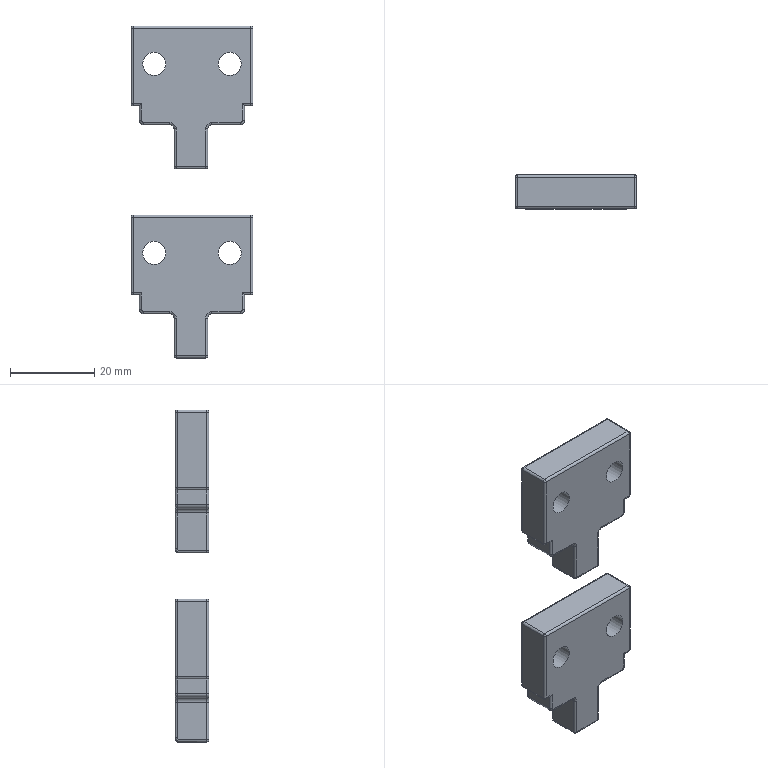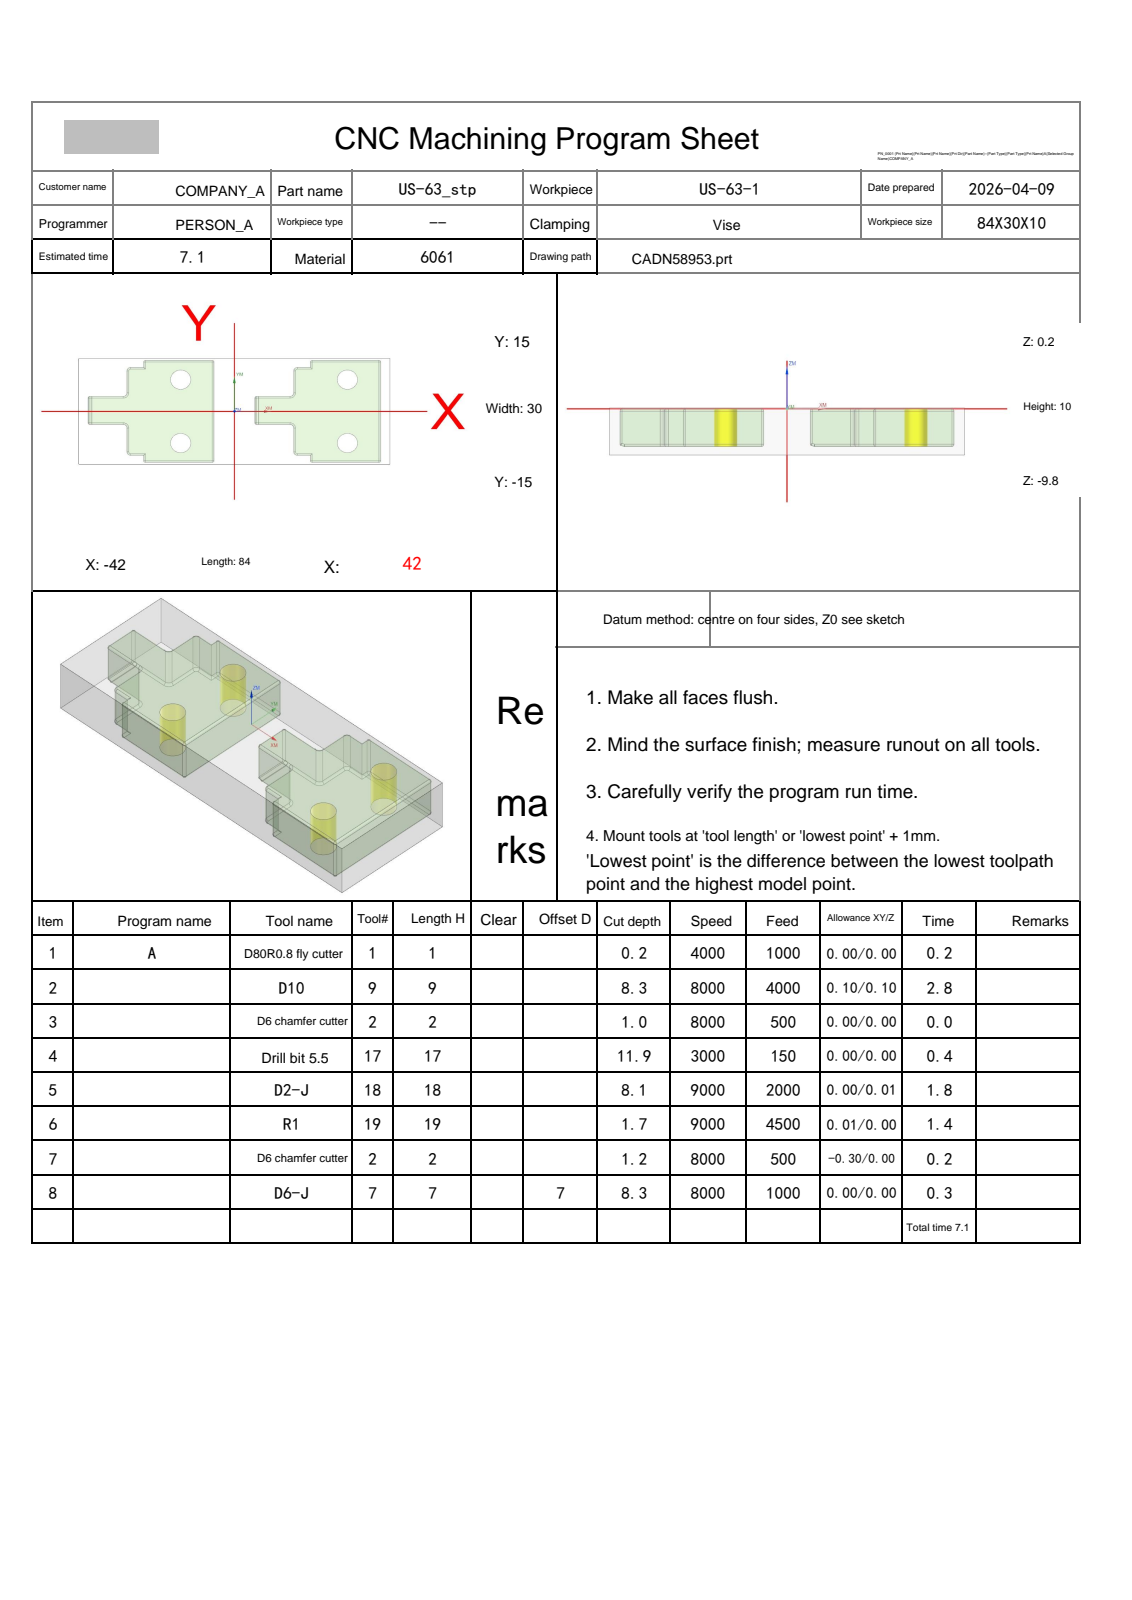NC program | NX | posted by the shop | part box 29 x 8 x 79 mm
Lines 34 to 1139 of 24039:
N2 T09 M06
(D10  D=10. R=0. H=09 ce=0.10 di=0.10)
G00 G90 G54 X12.55 Y-27. M03 S8000
G43 H09 Z10.2
M08
Z.724
G01 Z-.476 F4000.
Y-22.5
G03 X5.55 Y-15.5 I-7. J0.0
G01 X.837
G02 X-2.395 Y-20. I-6.837 J1.5
G01 X-27.605
G02 X-28.961 Y-18.938 I3.605 J6.
X-34.344 Y-15.5 I.961 J7.438
G01 X-42.
G02 X-42.5 Y-15. I0.0 J.5
G01 Y-10.535
G02 X-41.5 Y-9.535 I1. J0.0
X-41.214 Y-9.576 I0.0 J-1.
G01 X-39.39 Y-10.12
G03 X-38.298 Y-10.28 I1.092 J3.664
X-37.744 Y-10.239 I0.0 J3.824
G01 X-37.701 Y-10.236
X-35.798
G02 X-35.5 Y-10.535 I-.001 J-.3
G01 Y-10.701
G02 X-35.798 Y-11. I-.3 J.001
G01 X-37.701
X-37.79 Y-11.028
X-37.852 Y-10.958
G03 X-38.36 Y-10.82 I-.508 J-.862
X-38.599 Y-10.849 I0.0 J-1.
G01 X-41.26 Y-11.506
G02 X-41.5 Y-11.535 I-.24 J.971
X-42.5 Y-10.535 I0.0 J1.
G01 Y-9.298
G02 X-46. Y-3.236 I3.5 J6.062
G01 X-45.999 Y3.814
G02 X-42.5 Y9.825 I6.999 J-.05
G01 Y15.
G02 X-42. Y15.5 I.5 J0.0
G01 X-34.344
G02 X-28.961 Y18.938 I6.344 J-4.
X-27.605 Y20. I4.961 J-4.938
G01 X-2.395
G02 X.837 Y15.5 I-3.605 J-6.
G01 X4.477
G02 X5.477 Y14.5 I0.0 J-1.
X5.435 Y14.214 I-1. J0.0
G01 X4.831 Y12.187
G03 X4.667 Y11.066 I3.761 J-1.121
X4.675 Y10.813 I3.924 J0.0
G01 X4.676 Y10.8
G02 X4.519 Y10.605 I-.2 J0.0
G03 X2.089 Y9.569 I1.481 J-6.841
G02 X1.7 Y9.45 I-.39 J.582
X1. Y10.149 I0.0 J.7
G01 Y10.302
G02 X1.621 Y10.996 I.7 J-.002
G03 X2.454 Y11.666 I-.113 J.994
G01 X3.53 Y14.823
G02 X4.477 Y15.5 I.946 J-.323
G01 X10.656
G02 X16.039 Y18.938 I6.344 J-4.
X17.395 Y20. I4.961 J-4.938
G01 X42.
G02 X42.681 Y19.953 I0.0 J-5.
X46. Y14. I-3.681 J-5.953
G01 Y-14.
G02 X42.681 Y-19.953 I-7. J0.0
X42. Y-20. I-.681 J4.953
G01 X17.395
G02 X16.039 Y-18.938 I3.605 J6.
X10.656 Y-15.5 I.961 J7.438
G01 X.837
G02 X.77 Y-15.779 I-6.837 J1.5
X.417 Y-16.051 I-.353 J.093
X.052 Y-15.687 I0.0 J.365
G01 X.063 Y-15.596
X1.196 Y-11.178
G03 X1.223 Y-10.961 I-.844 J.216
X1.113 Y-10.538 I-.871 J0.0
G02 X1.003 Y-10.173 I.786 J.438
G03 X.812 Y-9.897 I-.335 J-.028
G01 X.2 Y-9.607
X.02 Y-9.566
G03 X-.4 Y-9.986 I0.0 J-.42
G01 Y-14.
G02 X-6. Y-19.6 I-5.6 J0.0
G01 X-24.
G02 X-28.295 Y-17.592 I0.0 J5.6
X-34.1 Y-11.5 I.295 J6.092
G01 Y-8.836
X-39.
G02 X-44.6 Y-3.236 I0.0 J5.6
G01 X-44.599 Y3.804
G02 X-39. Y9.363 I5.599 J-.04
G01 X-34.1
Y11.5
G02 X-28.295 Y17.592 I6.1 J0.0
X-24. Y19.6 I4.295 J-3.592
G01 X-6.
G02 X-.4 Y14. I0.0 J-5.6
G01 Y-9.986
G03 X.02 Y-10.406 I.42 J0.0
G01 X.2 Y-10.366
X.799 Y-10.081
G03 X1.019 Y-9.803 I-.172 J.361
G02 X1.9 Y-9.088 I.881 J-.186
X2.365 Y-9.218 I0.0 J-.9
G03 X6. Y-10.236 I3.635 J5.982
G01 X9.202
G02 X9.484 Y-10.437 I-.001 J-.3
G03 X9.885 Y-10.884 I.735 J.257
G01 X10.3 Y-11.081
X10.48 Y-11.121
G03 X10.9 Y-10.701 I0.0 J.42
G01 Y-8.836
X6.
G02 X.4 Y-3.236 I0.0 J5.6
G01 Y3.764
G02 X6. Y9.363 I5.6 J0.0
G01 X10.9
Y11.5
G02 X16.705 Y17.592 I6.1 J0.0
X21. Y19.6 I4.295 J-3.592
G01 X39.
G02 X44.6 Y14. I0.0 J-5.6
G01 Y-14.
G02 X39. Y-19.6 I-5.6 J0.0
G01 X21.
G02 X16.705 Y-17.592 I0.0 J5.6
X10.9 Y-11.5 I.295 J6.092
G01 Y-10.701
G03 X10.48 Y-10.281 I-.42 J0.0
G01 X10.3 Y-10.322
X9.669 Y-10.621
G03 X9.475 Y-10.821 I.172 J-.361
G02 X9.202 Y-11. I-.275 J.121
G01 X1.898
X1.724 Y-10.983
G02 X1.285 Y-10.757 I.176 J.883
G01 Z.724
G00 Z3.
G01 X12.55 Y-27. F6000.
G00 Z.247
G01 Z-.953 F4000.
Y-22.5
G03 X5.55 Y-15.5 I-7. J0.0
G01 X.837
G02 X-2.394 Y-20. I-6.837 J1.5
G01 X-27.606
G02 X-28.961 Y-18.938 I3.606 J6.
X-34.344 Y-15.5 I.961 J7.438
G01 X-42.
G02 X-42.5 Y-15. I0.0 J.5
G01 Y-10.535
G02 X-41.5 Y-9.535 I1. J0.0
X-41.214 Y-9.577 I0.0 J-1.
G01 X-39.39 Y-10.121
G03 X-38.298 Y-10.28 I1.092 J3.663
X-37.744 Y-10.24 I0.0 J3.823
G01 X-37.701 Y-10.236
X-35.799
G02 X-35.5 Y-10.535 I-.001 J-.3
G01 Y-10.701
G02 X-35.799 Y-11. I-.3 J.001
G01 X-37.701
X-37.79 Y-11.028
X-37.852 Y-10.958
G03 X-38.36 Y-10.82 I-.508 J-.862
X-38.599 Y-10.849 I0.0 J-1.
G01 X-41.26 Y-11.506
G02 X-41.5 Y-11.535 I-.24 J.971
X-42.5 Y-10.535 I0.0 J1.
G01 Y-9.299
G02 X-46. Y-3.236 I3.5 J6.062
G01 Y3.764
G02 X-42.5 Y9.826 I7. J0.0
G01 Y15.
G02 X-42. Y15.5 I.5 J0.0
G01 X-34.344
G02 X-28.961 Y18.938 I6.344 J-4.
X-27.606 Y20. I4.961 J-4.938
G01 X-2.394
G02 X.837 Y15.5 I-3.606 J-6.
G01 X4.475
G02 X5.475 Y14.5 I0.0 J-1.
X5.433 Y14.214 I-1. J0.0
G01 X4.828 Y12.187
G03 X4.665 Y11.067 I3.758 J-1.12
X4.673 Y10.813 I3.922 J0.0
G01 X4.674 Y10.8
G02 X4.517 Y10.605 I-.2 J0.0
G03 X2.09 Y9.57 I1.483 J-6.841
G02 X1.7 Y9.451 I-.39 J.582
X1. Y10.149 I0.0 J.7
G01 Y10.302
G02 X1.62 Y10.995 I.7 J-.002
G03 X2.452 Y11.666 I-.115 J.993
G01 X3.528 Y14.823
G02 X4.475 Y15.5 I.946 J-.323
G01 X10.656
G02 X16.039 Y18.938 I6.344 J-4.
X17.394 Y20. I4.961 J-4.938
G01 X42.
G02 X42.682 Y19.953 I0.0 J-5.
X46. Y14. I-3.682 J-5.953
G01 Y-14.
G02 X42.682 Y-19.953 I-7. J0.0
X42. Y-20. I-.682 J4.953
G01 X17.394
G02 X16.039 Y-18.938 I3.606 J6.
X10.656 Y-15.5 I.961 J7.438
G01 X.837
G02 X.77 Y-15.78 I-6.837 J1.5
X.417 Y-16.052 I-.353 J.093
X.052 Y-15.687 I0.0 J.365
G01 X.064 Y-15.596
X1.197 Y-11.178
G03 X1.224 Y-10.962 I-.844 J.216
X1.114 Y-10.538 I-.871 J0.0
G02 X1.003 Y-10.174 I.786 J.438
G03 X.813 Y-9.898 I-.334 J-.028
G01 X.2 Y-9.608
X.02 Y-9.567
G03 X-.4 Y-9.987 I0.0 J-.42
G01 Y-14.
G02 X-6. Y-19.6 I-5.6 J0.0
G01 X-24.
G02 X-28.296 Y-17.593 I0.0 J5.6
X-34.1 Y-11.5 I.296 J6.093
G01 Y-8.836
X-39.
G02 X-44.6 Y-3.236 I0.0 J5.6
G01 Y3.764
G02 X-39. Y9.364 I5.6 J0.0
G01 X-34.1
Y11.5
G02 X-28.296 Y17.593 I6.1 J0.0
X-24. Y19.6 I4.296 J-3.593
G01 X-6.
G02 X-.4 Y14. I0.0 J-5.6
G01 Y-9.987
G03 X.02 Y-10.407 I.42 J0.0
G01 X.2 Y-10.367
X.8 Y-10.082
G03 X1.019 Y-9.804 I-.172 J.361
G02 X1.9 Y-9.089 I.881 J-.186
X2.366 Y-9.219 I0.0 J-.9
G03 X6. Y-10.236 I3.634 J5.983
G01 X9.201
G02 X9.483 Y-10.437 I-.001 J-.3
G03 X9.884 Y-10.883 I.735 J.258
G01 X10.3 Y-11.081
X10.48 Y-11.121
G03 X10.9 Y-10.701 I0.0 J.42
G01 Y-8.836
X6.
G02 X.4 Y-3.236 I0.0 J5.6
G01 Y3.764
G02 X6. Y9.364 I5.6 J0.0
G01 X10.9
Y11.5
G02 X16.704 Y17.593 I6.1 J0.0
X21. Y19.6 I4.296 J-3.593
G01 X39.
G02 X44.6 Y14. I0.0 J-5.6
G01 Y-14.
G02 X39. Y-19.6 I-5.6 J0.0
G01 X21.
G02 X16.704 Y-17.593 I0.0 J5.6
X10.9 Y-11.5 I.296 J6.093
G01 Y-10.701
G03 X10.48 Y-10.281 I-.42 J0.0
G01 X10.3 Y-10.322
X9.669 Y-10.621
G03 X9.475 Y-10.821 I.172 J-.361
G02 X9.201 Y-11. I-.275 J.121
G01 X1.898
X1.724 Y-10.983
G02 X1.285 Y-10.757 I.176 J.883
G01 Z.247
G00 Z2.524
G01 X12.55 Y-27. F6000.
G00 Z-.229
G01 Z-1.429 F4000.
Y-22.5
G03 X5.55 Y-15.5 I-7. J0.0
G01 X.837
G02 X-2.394 Y-20. I-6.837 J1.5
G01 X-27.606
G02 X-28.961 Y-18.938 I3.606 J6.
X-34.344 Y-15.5 I.961 J7.438
G01 X-42.
G02 X-42.5 Y-15. I0.0 J.5
G01 Y-10.535
G02 X-41.5 Y-9.535 I1. J0.0
X-41.214 Y-9.577 I0.0 J-1.
G01 X-39.39 Y-10.121
G03 X-38.298 Y-10.28 I1.092 J3.663
X-37.744 Y-10.24 I0.0 J3.822
G01 X-37.701 Y-10.236
X-35.799
G02 X-35.5 Y-10.535 I-.001 J-.3
G01 Y-10.701
G02 X-35.799 Y-11. I-.3 J.001
G01 X-37.701
X-37.79 Y-11.028
X-37.852 Y-10.958
G03 X-38.36 Y-10.82 I-.507 J-.862
X-38.599 Y-10.849 I0.0 J-1.
G01 X-41.26 Y-11.506
G02 X-41.5 Y-11.535 I-.24 J.971
X-42.5 Y-10.535 I0.0 J1.
G01 Y-9.299
G02 X-46. Y-3.236 I3.5 J6.062
G01 Y3.764
G02 X-42.5 Y9.826 I7. J0.0
G01 Y15.
G02 X-42. Y15.5 I.5 J0.0
G01 X-34.344
G02 X-28.961 Y18.938 I6.344 J-4.
X-27.606 Y20. I4.961 J-4.938
G01 X-2.394
G02 X.837 Y15.5 I-3.606 J-6.
G01 X4.475
G02 X5.475 Y14.5 I0.0 J-1.
X5.433 Y14.214 I-1. J0.0
G01 X4.828 Y12.186
G03 X4.665 Y11.066 I3.758 J-1.12
X4.673 Y10.813 I3.922 J0.0
G01 X4.674 Y10.8
G02 X4.517 Y10.605 I-.2 J0.0
G03 X2.089 Y9.569 I1.483 J-6.841
G02 X1.7 Y9.451 I-.389 J.582
X1. Y10.149 I0.0 J.7
G01 Y10.302
G02 X1.62 Y10.995 I.7 J-.002
G03 X2.452 Y11.666 I-.115 J.993
G01 X3.528 Y14.823
G02 X4.475 Y15.5 I.946 J-.323
G01 X10.656
G02 X16.039 Y18.938 I6.344 J-4.
X17.394 Y20. I4.961 J-4.938
G01 X42.
G02 X42.682 Y19.953 I0.0 J-5.
X46. Y14. I-3.682 J-5.953
G01 Y-14.
G02 X42.682 Y-19.953 I-7. J0.0
X42. Y-20. I-.682 J4.953
G01 X17.394
G02 X16.039 Y-18.938 I3.606 J6.
X10.656 Y-15.5 I.961 J7.438
G01 X.837
G02 X.77 Y-15.78 I-6.837 J1.5
X.417 Y-16.052 I-.353 J.093
X.052 Y-15.687 I0.0 J.365
G01 X.064 Y-15.596
X1.197 Y-11.178
G03 X1.224 Y-10.962 I-.844 J.216
X1.114 Y-10.538 I-.871 J0.0
G02 X1.003 Y-10.174 I.786 J.438
G03 X.813 Y-9.898 I-.334 J-.028
G01 X.2 Y-9.608
X.02 Y-9.567
G03 X-.4 Y-9.987 I0.0 J-.42
G01 Y-14.
G02 X-6. Y-19.6 I-5.6 J0.0
G01 X-24.
G02 X-28.296 Y-17.593 I0.0 J5.6
X-34.1 Y-11.5 I.296 J6.093
G01 Y-8.836
X-39.
G02 X-44.6 Y-3.236 I0.0 J5.6
G01 Y3.764
G02 X-39. Y9.364 I5.6 J0.0
G01 X-34.1
Y11.5
G02 X-28.296 Y17.593 I6.1 J0.0
X-24. Y19.6 I4.296 J-3.593
G01 X-6.
G02 X-.4 Y14. I0.0 J-5.6
G01 Y-9.987
G03 X.02 Y-10.407 I.42 J0.0
G01 X.2 Y-10.366
X.8 Y-10.082
G03 X1.019 Y-9.803 I-.172 J.361
G02 X1.9 Y-9.089 I.881 J-.186
X2.365 Y-9.219 I0.0 J-.9
G03 X6. Y-10.236 I3.635 J5.982
G01 X9.201
G02 X9.483 Y-10.437 I-.001 J-.3
G03 X9.884 Y-10.884 I.735 J.258
G01 X10.3 Y-11.081
X10.48 Y-11.121
G03 X10.9 Y-10.701 I0.0 J.42
G01 Y-8.836
X6.
G02 X.4 Y-3.236 I0.0 J5.6
G01 Y3.764
G02 X6. Y9.364 I5.6 J0.0
G01 X10.9
Y11.5
G02 X16.704 Y17.593 I6.1 J0.0
X21. Y19.6 I4.296 J-3.593
G01 X39.
G02 X44.6 Y14. I0.0 J-5.6
G01 Y-14.
G02 X39. Y-19.6 I-5.6 J0.0
G01 X21.
G02 X16.704 Y-17.593 I0.0 J5.6
X10.9 Y-11.5 I.296 J6.093
G01 Y-10.701
G03 X10.48 Y-10.281 I-.42 J0.0
G01 X10.3 Y-10.322
X9.669 Y-10.621
G03 X9.475 Y-10.821 I.172 J-.361
G02 X9.201 Y-11. I-.275 J.121
G01 X1.898
X1.724 Y-10.983
G02 X1.285 Y-10.757 I.176 J.883
G01 Z-.229
G00 Z2.047
G01 X12.55 Y-27. F6000.
G00 Z-.706
G01 Z-1.906 F4000.
Y-22.5
G03 X5.55 Y-15.5 I-7. J0.0
G01 X.837
G02 X-2.394 Y-20. I-6.837 J1.5
G01 X-27.606
G02 X-28.961 Y-18.938 I3.606 J6.
X-34.344 Y-15.5 I.961 J7.438
G01 X-42.
G02 X-42.5 Y-15. I0.0 J.5
G01 Y-10.535
G02 X-41.5 Y-9.535 I1. J0.0
X-41.214 Y-9.577 I0.0 J-1.
G01 X-39.39 Y-10.121
G03 X-38.298 Y-10.28 I1.092 J3.663
X-37.744 Y-10.24 I0.0 J3.823
G01 X-37.701 Y-10.236
X-35.799
G02 X-35.5 Y-10.535 I-.001 J-.3
G01 Y-10.701
G02 X-35.799 Y-11. I-.3 J.001
G01 X-37.701
X-37.79 Y-11.028
X-37.852 Y-10.958
G03 X-38.36 Y-10.82 I-.508 J-.862
X-38.599 Y-10.849 I0.0 J-1.
G01 X-41.26 Y-11.506
G02 X-41.5 Y-11.535 I-.24 J.971
X-42.5 Y-10.535 I0.0 J1.
G01 Y-9.299
G02 X-46. Y-3.236 I3.5 J6.062
G01 Y3.764
G02 X-42.5 Y9.826 I7. J0.0
G01 Y15.
G02 X-42. Y15.5 I.5 J0.0
G01 X-34.344
G02 X-28.961 Y18.938 I6.344 J-4.
X-27.606 Y20. I4.961 J-4.938
G01 X-2.394
G02 X.837 Y15.5 I-3.606 J-6.
G01 X4.475
G02 X5.475 Y14.5 I0.0 J-1.
X5.433 Y14.214 I-1. J0.0
G01 X4.828 Y12.187
G03 X4.665 Y11.067 I3.758 J-1.12
X4.673 Y10.813 I3.922 J0.0
G01 X4.674 Y10.8
G02 X4.517 Y10.605 I-.2 J0.0
G03 X2.09 Y9.57 I1.483 J-6.841
G02 X1.7 Y9.451 I-.39 J.582
X1. Y10.149 I0.0 J.7
G01 Y10.302
G02 X1.62 Y10.995 I.7 J-.002
G03 X2.452 Y11.666 I-.115 J.993
G01 X3.528 Y14.823
G02 X4.475 Y15.5 I.946 J-.323
G01 X10.656
G02 X16.039 Y18.938 I6.344 J-4.
X17.394 Y20. I4.961 J-4.938
G01 X42.
G02 X42.682 Y19.953 I0.0 J-5.
X46. Y14. I-3.682 J-5.953
G01 Y-14.
G02 X42.682 Y-19.953 I-7. J0.0
X42. Y-20. I-.682 J4.953
G01 X17.394
G02 X16.039 Y-18.938 I3.606 J6.
X10.656 Y-15.5 I.961 J7.438
G01 X.837
G02 X.77 Y-15.78 I-6.837 J1.5
X.417 Y-16.052 I-.353 J.093
X.052 Y-15.687 I0.0 J.365
G01 X.064 Y-15.596
X1.197 Y-11.178
G03 X1.224 Y-10.962 I-.844 J.216
X1.114 Y-10.538 I-.871 J0.0
G02 X1.003 Y-10.174 I.786 J.438
G03 X.813 Y-9.898 I-.334 J-.028
G01 X.2 Y-9.608
X.02 Y-9.567
G03 X-.4 Y-9.987 I0.0 J-.42
G01 Y-14.
G02 X-6. Y-19.6 I-5.6 J0.0
G01 X-24.
G02 X-28.296 Y-17.593 I0.0 J5.6
X-34.1 Y-11.5 I.296 J6.093
G01 Y-8.836
X-39.
G02 X-44.6 Y-3.236 I0.0 J5.6
G01 Y3.764
G02 X-39. Y9.364 I5.6 J0.0
G01 X-34.1
Y11.5
G02 X-28.296 Y17.593 I6.1 J0.0
X-24. Y19.6 I4.296 J-3.593
G01 X-6.
G02 X-.4 Y14. I0.0 J-5.6
G01 Y-9.987
G03 X.02 Y-10.407 I.42 J0.0
G01 X.2 Y-10.367
X.8 Y-10.082
G03 X1.019 Y-9.804 I-.172 J.361
G02 X1.9 Y-9.089 I.881 J-.186
X2.366 Y-9.219 I0.0 J-.9
G03 X6. Y-10.236 I3.634 J5.983
G01 X9.201
G02 X9.483 Y-10.437 I-.001 J-.3
G03 X9.884 Y-10.883 I.735 J.258
G01 X10.3 Y-11.081
X10.48 Y-11.121
G03 X10.9 Y-10.701 I0.0 J.42
G01 Y-8.836
X6.
G02 X.4 Y-3.236 I0.0 J5.6
G01 Y3.764
G02 X6. Y9.364 I5.6 J0.0
G01 X10.9
Y11.5
G02 X16.704 Y17.593 I6.1 J0.0
X21. Y19.6 I4.296 J-3.593
G01 X39.
G02 X44.6 Y14. I0.0 J-5.6
G01 Y-14.
G02 X39. Y-19.6 I-5.6 J0.0
G01 X21.
G02 X16.704 Y-17.593 I0.0 J5.6
X10.9 Y-11.5 I.296 J6.093
G01 Y-10.701
G03 X10.48 Y-10.281 I-.42 J0.0
G01 X10.3 Y-10.322
X9.669 Y-10.621
G03 X9.475 Y-10.821 I.172 J-.361
G02 X9.201 Y-11. I-.275 J.121
G01 X1.898
X1.724 Y-10.983
G02 X1.285 Y-10.757 I.176 J.883
G01 Z-.706
G00 Z1.571
G01 X12.55 Y-27. F6000.
G00 Z-1.182
G01 Z-2.382 F4000.
Y-22.5
G03 X5.55 Y-15.5 I-7. J0.0
G01 X.837
G02 X-2.394 Y-20. I-6.837 J1.5
G01 X-27.606
G02 X-28.961 Y-18.938 I3.606 J6.
X-34.344 Y-15.5 I.961 J7.438
G01 X-42.
G02 X-42.5 Y-15. I0.0 J.5
G01 Y-10.535
G02 X-41.5 Y-9.535 I1. J0.0
X-41.214 Y-9.577 I0.0 J-1.
G01 X-39.39 Y-10.121
G03 X-38.298 Y-10.28 I1.092 J3.663
X-37.744 Y-10.24 I0.0 J3.822
G01 X-37.701 Y-10.236
X-35.799
G02 X-35.5 Y-10.535 I-.001 J-.3
G01 Y-10.701
G02 X-35.799 Y-11. I-.3 J.001
G01 X-37.701
X-37.79 Y-11.028
X-37.852 Y-10.958
G03 X-38.36 Y-10.82 I-.507 J-.862
X-38.599 Y-10.849 I0.0 J-1.
G01 X-41.26 Y-11.506
G02 X-41.5 Y-11.535 I-.24 J.971
X-42.5 Y-10.535 I0.0 J1.
G01 Y-9.299
G02 X-46. Y-3.236 I3.5 J6.062
G01 Y3.764
G02 X-42.5 Y9.826 I7. J0.0
G01 Y15.
G02 X-42. Y15.5 I.5 J0.0
G01 X-34.344
G02 X-28.961 Y18.938 I6.344 J-4.
X-27.606 Y20. I4.961 J-4.938
G01 X-2.394
G02 X.837 Y15.5 I-3.606 J-6.
G01 X4.475
G02 X5.475 Y14.5 I0.0 J-1.
X5.433 Y14.214 I-1. J0.0
G01 X4.828 Y12.186
G03 X4.665 Y11.066 I3.758 J-1.12
X4.673 Y10.813 I3.922 J0.0
G01 X4.674 Y10.8
G02 X4.517 Y10.605 I-.2 J0.0
G03 X2.089 Y9.569 I1.483 J-6.841
G02 X1.7 Y9.451 I-.389 J.582
X1. Y10.149 I0.0 J.7
G01 Y10.302
G02 X1.62 Y10.995 I.7 J-.002
G03 X2.452 Y11.666 I-.115 J.993
G01 X3.528 Y14.823
G02 X4.475 Y15.5 I.946 J-.323
G01 X10.656
G02 X16.039 Y18.938 I6.344 J-4.
X17.394 Y20. I4.961 J-4.938
G01 X42.
G02 X42.682 Y19.953 I0.0 J-5.
X46. Y14. I-3.682 J-5.953
G01 Y-14.
G02 X42.682 Y-19.953 I-7. J0.0
X42. Y-20. I-.682 J4.953
G01 X17.394
G02 X16.039 Y-18.938 I3.606 J6.
X10.656 Y-15.5 I.961 J7.438
G01 X.837
G02 X.77 Y-15.78 I-6.837 J1.5
X.417 Y-16.052 I-.353 J.093
X.052 Y-15.687 I0.0 J.365
G01 X.064 Y-15.596
X1.197 Y-11.178
G03 X1.224 Y-10.962 I-.844 J.216
X1.114 Y-10.538 I-.871 J0.0
G02 X1.003 Y-10.174 I.786 J.438
G03 X.813 Y-9.898 I-.334 J-.028
G01 X.2 Y-9.608
X.02 Y-9.567
G03 X-.4 Y-9.987 I0.0 J-.42
G01 Y-14.
G02 X-6. Y-19.6 I-5.6 J0.0
G01 X-24.
G02 X-28.296 Y-17.593 I0.0 J5.6
X-34.1 Y-11.5 I.296 J6.093
G01 Y-8.836
X-39.
G02 X-44.6 Y-3.236 I0.0 J5.6
G01 Y3.764
G02 X-39. Y9.364 I5.6 J0.0
G01 X-34.1
Y11.5
G02 X-28.296 Y17.593 I6.1 J0.0
X-24. Y19.6 I4.296 J-3.593
G01 X-6.
G02 X-.4 Y14. I0.0 J-5.6
G01 Y-9.987
G03 X.02 Y-10.407 I.42 J0.0
G01 X.2 Y-10.366
X.8 Y-10.082
G03 X1.019 Y-9.803 I-.172 J.361
G02 X1.9 Y-9.089 I.881 J-.186
X2.365 Y-9.219 I0.0 J-.9
G03 X6. Y-10.236 I3.635 J5.982
G01 X9.201
G02 X9.483 Y-10.437 I-.001 J-.3
G03 X9.884 Y-10.884 I.735 J.258
G01 X10.3 Y-11.081
X10.48 Y-11.121
G03 X10.9 Y-10.701 I0.0 J.42
G01 Y-8.836
X6.
G02 X.4 Y-3.236 I0.0 J5.6
G01 Y3.764
G02 X6. Y9.364 I5.6 J0.0
G01 X10.9
Y11.5
G02 X16.704 Y17.593 I6.1 J0.0
X21. Y19.6 I4.296 J-3.593
G01 X39.
G02 X44.6 Y14. I0.0 J-5.6
G01 Y-14.
G02 X39. Y-19.6 I-5.6 J0.0
G01 X21.
G02 X16.704 Y-17.593 I0.0 J5.6
X10.9 Y-11.5 I.296 J6.093
G01 Y-10.701
G03 X10.48 Y-10.281 I-.42 J0.0
G01 X10.3 Y-10.322
X9.669 Y-10.621
G03 X9.475 Y-10.821 I.172 J-.361
G02 X9.201 Y-11. I-.275 J.121
G01 X1.898
X1.724 Y-10.983
G02 X1.285 Y-10.757 I.176 J.883
G01 Z-1.182
G00 Z1.094
G01 X12.55 Y-27. F6000.
G00 Z-1.659
G01 Z-2.859 F4000.
Y-22.5
G03 X5.55 Y-15.5 I-7. J0.0
G01 X.837
G02 X-2.394 Y-20. I-6.837 J1.5
G01 X-27.606
G02 X-28.961 Y-18.938 I3.606 J6.
X-34.344 Y-15.5 I.961 J7.438
G01 X-42.
G02 X-42.5 Y-15. I0.0 J.5
G01 Y-10.535
G02 X-41.5 Y-9.535 I1. J0.0
X-41.214 Y-9.577 I0.0 J-1.
G01 X-39.39 Y-10.121
G03 X-38.298 Y-10.28 I1.092 J3.663
X-37.744 Y-10.24 I0.0 J3.823
G01 X-37.701 Y-10.236
X-35.799
G02 X-35.5 Y-10.535 I-.001 J-.3
G01 Y-10.701
G02 X-35.799 Y-11. I-.3 J.001
G01 X-37.701
X-37.79 Y-11.028
X-37.852 Y-10.958
G03 X-38.36 Y-10.82 I-.508 J-.862
X-38.599 Y-10.849 I0.0 J-1.
G01 X-41.26 Y-11.506
G02 X-41.5 Y-11.535 I-.24 J.971
X-42.5 Y-10.535 I0.0 J1.
G01 Y-9.299
G02 X-46. Y-3.236 I3.5 J6.062
G01 Y3.764
G02 X-42.5 Y9.826 I7. J0.0
G01 Y15.
G02 X-42. Y15.5 I.5 J0.0
G01 X-34.344
G02 X-28.961 Y18.938 I6.344 J-4.
X-27.606 Y20. I4.961 J-4.938
G01 X-2.394
G02 X.837 Y15.5 I-3.606 J-6.
G01 X4.475
G02 X5.475 Y14.5 I0.0 J-1.
X5.433 Y14.214 I-1. J0.0
G01 X4.828 Y12.187
G03 X4.665 Y11.067 I3.758 J-1.12
X4.673 Y10.813 I3.922 J0.0
G01 X4.674 Y10.8
G02 X4.517 Y10.605 I-.2 J0.0
G03 X2.09 Y9.57 I1.483 J-6.841
G02 X1.7 Y9.451 I-.39 J.582
X1. Y10.149 I0.0 J.7
G01 Y10.302
G02 X1.62 Y10.995 I.7 J-.002
G03 X2.452 Y11.666 I-.115 J.993
G01 X3.528 Y14.823
G02 X4.475 Y15.5 I.946 J-.323
G01 X10.656
G02 X16.039 Y18.938 I6.344 J-4.
X17.394 Y20. I4.961 J-4.938
G01 X42.
G02 X42.682 Y19.953 I0.0 J-5.
X46. Y14. I-3.682 J-5.953
G01 Y-14.
G02 X42.682 Y-19.953 I-7. J0.0
X42. Y-20. I-.682 J4.953
G01 X17.394
G02 X16.039 Y-18.938 I3.606 J6.
X10.656 Y-15.5 I.961 J7.438
G01 X.837
G02 X.77 Y-15.78 I-6.837 J1.5
X.417 Y-16.052 I-.353 J.093
X.052 Y-15.687 I0.0 J.365
G01 X.064 Y-15.596
X1.197 Y-11.178
G03 X1.224 Y-10.962 I-.844 J.216
X1.114 Y-10.538 I-.871 J0.0
G02 X1.003 Y-10.174 I.786 J.438
G03 X.813 Y-9.898 I-.334 J-.028
G01 X.2 Y-9.608
X.02 Y-9.567
G03 X-.4 Y-9.987 I0.0 J-.42
G01 Y-14.
G02 X-6. Y-19.6 I-5.6 J0.0
G01 X-24.
G02 X-28.296 Y-17.593 I0.0 J5.6
X-34.1 Y-11.5 I.296 J6.093
G01 Y-8.836
X-39.
G02 X-44.6 Y-3.236 I0.0 J5.6
G01 Y3.764
G02 X-39. Y9.364 I5.6 J0.0
G01 X-34.1
Y11.5
G02 X-28.296 Y17.593 I6.1 J0.0
X-24. Y19.6 I4.296 J-3.593
G01 X-6.
G02 X-.4 Y14. I0.0 J-5.6
G01 Y-9.987
G03 X.02 Y-10.407 I.42 J0.0
G01 X.2 Y-10.367
X.8 Y-10.082
G03 X1.019 Y-9.804 I-.172 J.361
G02 X1.9 Y-9.089 I.881 J-.186
X2.366 Y-9.219 I0.0 J-.9
G03 X6. Y-10.236 I3.634 J5.983
G01 X9.201
G02 X9.483 Y-10.437 I-.001 J-.3
G03 X9.884 Y-10.883 I.735 J.258
G01 X10.3 Y-11.081
X10.48 Y-11.121
G03 X10.9 Y-10.701 I0.0 J.42
G01 Y-8.836
X6.
G02 X.4 Y-3.236 I0.0 J5.6
G01 Y3.764
G02 X6. Y9.364 I5.6 J0.0
G01 X10.9
Y11.5
G02 X16.704 Y17.593 I6.1 J0.0
X21. Y19.6 I4.296 J-3.593
G01 X39.
G02 X44.6 Y14. I0.0 J-5.6
G01 Y-14.
G02 X39. Y-19.6 I-5.6 J0.0
G01 X21.
G02 X16.704 Y-17.593 I0.0 J5.6
X10.9 Y-11.5 I.296 J6.093
G01 Y-10.701
G03 X10.48 Y-10.281 I-.42 J0.0
G01 X10.3 Y-10.322
X9.669 Y-10.621
G03 X9.475 Y-10.821 I.172 J-.361
G02 X9.201 Y-11. I-.275 J.121
G01 X1.898
X1.724 Y-10.983
G02 X1.285 Y-10.757 I.176 J.883
G01 Z-1.659
G00 Z.618
G01 X12.55 Y-27. F6000.
G00 Z-2.135
G01 Z-3.335 F4000.
Y-22.5
G03 X5.55 Y-15.5 I-7. J0.0
G01 X.837
G02 X-2.394 Y-20. I-6.837 J1.5
G01 X-27.606
G02 X-28.961 Y-18.938 I3.606 J6.
X-34.344 Y-15.5 I.961 J7.438
G01 X-42.
G02 X-42.5 Y-15. I0.0 J.5
G01 Y-10.535
G02 X-41.5 Y-9.535 I1. J0.0
X-41.214 Y-9.577 I0.0 J-1.
G01 X-39.39 Y-10.121
G03 X-38.298 Y-10.28 I1.092 J3.663
X-37.744 Y-10.24 I0.0 J3.822
G01 X-37.701 Y-10.236
X-35.799
G02 X-35.5 Y-10.535 I-.001 J-.3
G01 Y-10.701
G02 X-35.799 Y-11. I-.3 J.001
G01 X-37.701
X-37.79 Y-11.028
X-37.852 Y-10.958
G03 X-38.36 Y-10.82 I-.507 J-.862
X-38.599 Y-10.849 I0.0 J-1.
G01 X-41.26 Y-11.506
G02 X-41.5 Y-11.535 I-.24 J.971
X-42.5 Y-10.535 I0.0 J1.
G01 Y-9.299
G02 X-46. Y-3.236 I3.5 J6.062
G01 Y3.764
G02 X-42.5 Y9.826 I7. J0.0
G01 Y15.
G02 X-42. Y15.5 I.5 J0.0
G01 X-34.344
G02 X-28.961 Y18.938 I6.344 J-4.
X-27.606 Y20. I4.961 J-4.938
G01 X-2.394
G02 X.837 Y15.5 I-3.606 J-6.
G01 X4.475
G02 X5.475 Y14.5 I0.0 J-1.
X5.433 Y14.214 I-1. J0.0
G01 X4.828 Y12.186
G03 X4.665 Y11.066 I3.758 J-1.12
X4.673 Y10.813 I3.922 J0.0
G01 X4.674 Y10.8
G02 X4.517 Y10.605 I-.2 J0.0
G03 X2.089 Y9.569 I1.483 J-6.841
G02 X1.7 Y9.451 I-.389 J.582
X1. Y10.149 I0.0 J.7
G01 Y10.302
G02 X1.62 Y10.995 I.7 J-.002
G03 X2.452 Y11.666 I-.115 J.993
G01 X3.528 Y14.823
G02 X4.475 Y15.5 I.946 J-.323
G01 X10.656
G02 X16.039 Y18.938 I6.344 J-4.
X17.394 Y20. I4.961 J-4.938
G01 X42.
G02 X42.682 Y19.953 I0.0 J-5.
X46. Y14. I-3.682 J-5.953
G01 Y-14.
G02 X42.682 Y-19.953 I-7. J0.0
X42. Y-20. I-.682 J4.953
G01 X17.394
G02 X16.039 Y-18.938 I3.606 J6.
X10.656 Y-15.5 I.961 J7.438
G01 X.837
G02 X.77 Y-15.78 I-6.837 J1.5
X.417 Y-16.052 I-.353 J.093
X.052 Y-15.687 I0.0 J.365
G01 X.064 Y-15.596
X1.197 Y-11.178
G03 X1.224 Y-10.962 I-.844 J.216
X1.114 Y-10.538 I-.871 J0.0
G02 X1.003 Y-10.174 I.786 J.438
G03 X.813 Y-9.898 I-.334 J-.028
G01 X.2 Y-9.608
X.02 Y-9.567
G03 X-.4 Y-9.987 I0.0 J-.42
G01 Y-14.
G02 X-6. Y-19.6 I-5.6 J0.0
G01 X-24.
G02 X-28.296 Y-17.593 I0.0 J5.6
X-34.1 Y-11.5 I.296 J6.093
G01 Y-8.836
X-39.
G02 X-44.6 Y-3.236 I0.0 J5.6
G01 Y3.764
G02 X-39. Y9.364 I5.6 J0.0
G01 X-34.1
Y11.5
G02 X-28.296 Y17.593 I6.1 J0.0
X-24. Y19.6 I4.296 J-3.593
G01 X-6.
G02 X-.4 Y14. I0.0 J-5.6
G01 Y-9.987
G03 X.02 Y-10.407 I.42 J0.0
G01 X.2 Y-10.366
X.8 Y-10.082
G03 X1.019 Y-9.803 I-.172 J.361
G02 X1.9 Y-9.089 I.881 J-.186
X2.365 Y-9.219 I0.0 J-.9
G03 X6. Y-10.236 I3.635 J5.982
G01 X9.201
G02 X9.483 Y-10.437 I-.001 J-.3
G03 X9.884 Y-10.884 I.735 J.258
G01 X10.3 Y-11.081
X10.48 Y-11.121
G03 X10.9 Y-10.701 I0.0 J.42
G01 Y-8.836
X6.
G02 X.4 Y-3.236 I0.0 J5.6
G01 Y3.764
G02 X6. Y9.364 I5.6 J0.0
G01 X10.9
Y11.5
G02 X16.704 Y17.593 I6.1 J0.0
X21. Y19.6 I4.296 J-3.593
G01 X39.
G02 X44.6 Y14. I0.0 J-5.6
G01 Y-14.
G02 X39. Y-19.6 I-5.6 J0.0
G01 X21.
G02 X16.704 Y-17.593 I0.0 J5.6
X10.9 Y-11.5 I.296 J6.093
G01 Y-10.701
G03 X10.48 Y-10.281 I-.42 J0.0
G01 X10.3 Y-10.322
X9.669 Y-10.621
G03 X9.475 Y-10.821 I.172 J-.361
G02 X9.201 Y-11. I-.275 J.121
G01 X1.898
X1.724 Y-10.983
G02 X1.285 Y-10.757 I.176 J.883
G01 Z-2.135
G00 Z.141
G01 X12.55 Y-27. F6000.
G00 Z-2.612
G01 Z-3.812 F4000.
Y-22.5
G03 X5.55 Y-15.5 I-7. J0.0
G01 X.837
G02 X-2.394 Y-20. I-6.837 J1.5
G01 X-27.606
G02 X-28.961 Y-18.938 I3.606 J6.
X-34.344 Y-15.5 I.961 J7.438
G01 X-42.
G02 X-42.5 Y-15. I0.0 J.5
G01 Y-10.535
G02 X-41.5 Y-9.535 I1. J0.0
X-41.214 Y-9.577 I0.0 J-1.
G01 X-39.39 Y-10.121
G03 X-38.298 Y-10.28 I1.092 J3.663
X-37.744 Y-10.24 I0.0 J3.823
G01 X-37.701 Y-10.236
X-35.799
G02 X-35.5 Y-10.535 I-.001 J-.3
G01 Y-10.701
G02 X-35.799 Y-11. I-.3 J.001
G01 X-37.701
X-37.79 Y-11.028
X-37.852 Y-10.958
G03 X-38.36 Y-10.82 I-.508 J-.862
X-38.599 Y-10.849 I0.0 J-1.
G01 X-41.26 Y-11.506
G02 X-41.5 Y-11.535 I-.24 J.971
X-42.5 Y-10.535 I0.0 J1.
G01 Y-9.299
G02 X-46. Y-3.236 I3.5 J6.062
G01 Y3.764
G02 X-42.5 Y9.826 I7. J0.0
G01 Y15.
G02 X-42. Y15.5 I.5 J0.0
G01 X-34.344
G02 X-28.961 Y18.938 I6.344 J-4.
X-27.606 Y20. I4.961 J-4.938
G01 X-2.394
G02 X.837 Y15.5 I-3.606 J-6.
G01 X4.475
G02 X5.475 Y14.5 I0.0 J-1.
X5.433 Y14.214 I-1. J0.0
G01 X4.828 Y12.187
G03 X4.665 Y11.067 I3.758 J-1.12
X4.673 Y10.813 I3.922 J0.0
G01 X4.674 Y10.8
G02 X4.517 Y10.605 I-.2 J0.0
G03 X2.09 Y9.57 I1.483 J-6.841
G02 X1.7 Y9.451 I-.39 J.582
X1. Y10.149 I0.0 J.7
G01 Y10.302
G02 X1.62 Y10.995 I.7 J-.002
G03 X2.452 Y11.666 I-.115 J.993
G01 X3.528 Y14.823
G02 X4.475 Y15.5 I.946 J-.323
G01 X10.656
G02 X16.039 Y18.938 I6.344 J-4.
X17.394 Y20. I4.961 J-4.938
G01 X42.
G02 X42.682 Y19.953 I0.0 J-5.
X46. Y14. I-3.682 J-5.953
G01 Y-14.
G02 X42.682 Y-19.953 I-7. J0.0
X42. Y-20. I-.682 J4.953
G01 X17.394
G02 X16.039 Y-18.938 I3.606 J6.
X10.656 Y-15.5 I.961 J7.438
G01 X.837
G02 X.77 Y-15.78 I-6.837 J1.5
X.417 Y-16.052 I-.353 J.093
X.052 Y-15.687 I0.0 J.365
G01 X.064 Y-15.596
X1.197 Y-11.178
G03 X1.224 Y-10.962 I-.844 J.216
X1.114 Y-10.538 I-.871 J0.0
G02 X1.003 Y-10.174 I.786 J.438
G03 X.813 Y-9.898 I-.334 J-.028
G01 X.2 Y-9.608
X.02 Y-9.567
G03 X-.4 Y-9.987 I0.0 J-.42
G01 Y-14.
G02 X-6. Y-19.6 I-5.6 J0.0
G01 X-24.
G02 X-28.296 Y-17.593 I0.0 J5.6
X-34.1 Y-11.5 I.296 J6.093
G01 Y-8.836
X-39.
G02 X-44.6 Y-3.236 I0.0 J5.6
G01 Y3.764
G02 X-39. Y9.364 I5.6 J0.0
G01 X-34.1
Y11.5
G02 X-28.296 Y17.593 I6.1 J0.0
X-24. Y19.6 I4.296 J-3.593
G01 X-6.
G02 X-.4 Y14. I0.0 J-5.6
G01 Y-9.987
G03 X.02 Y-10.407 I.42 J0.0
G01 X.2 Y-10.367
X.8 Y-10.082
G03 X1.019 Y-9.804 I-.172 J.361
G02 X1.9 Y-9.089 I.881 J-.186
X2.366 Y-9.219 I0.0 J-.9
G03 X6. Y-10.236 I3.634 J5.983
G01 X9.201
G02 X9.483 Y-10.437 I-.001 J-.3
G03 X9.884 Y-10.883 I.735 J.258
G01 X10.3 Y-11.081
X10.48 Y-11.121
G03 X10.9 Y-10.701 I0.0 J.42
G01 Y-8.836
X6.
G02 X.4 Y-3.236 I0.0 J5.6
G01 Y3.764
G02 X6. Y9.364 I5.6 J0.0
G01 X10.9
Y11.5
G02 X16.704 Y17.593 I6.1 J0.0
X21. Y19.6 I4.296 J-3.593